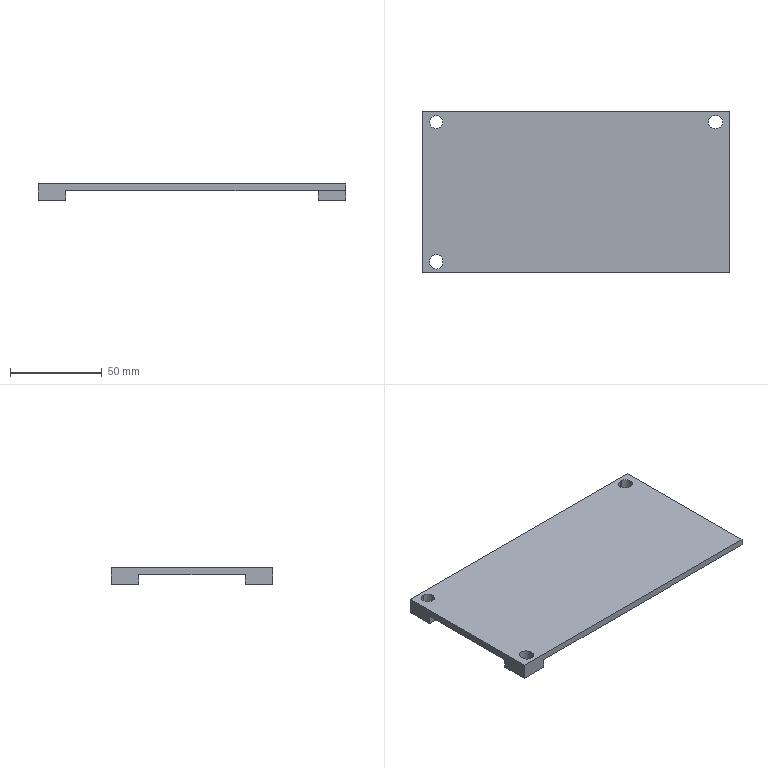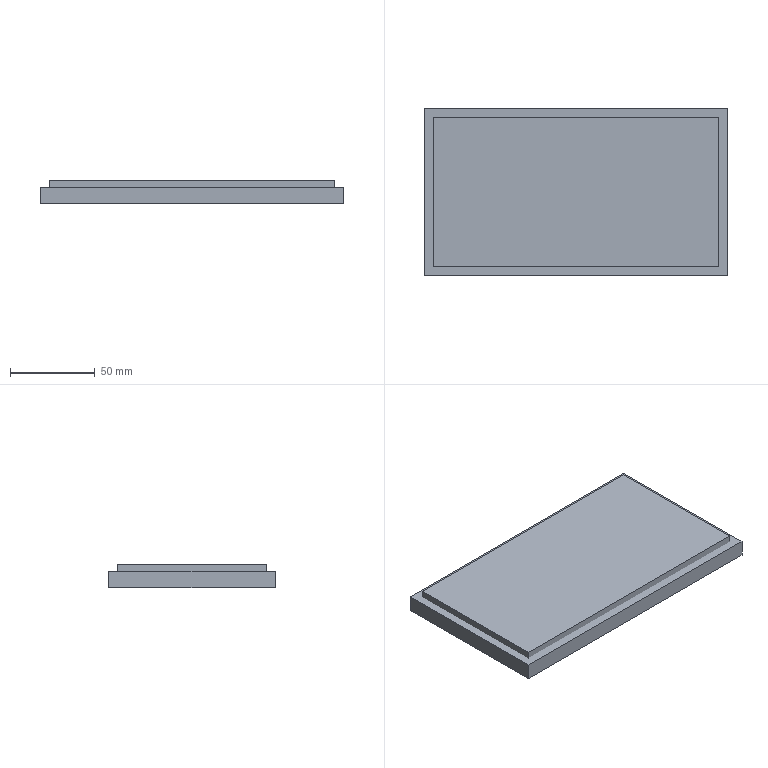CAM job | NX | 3-axis milling | part box 168 x 88.2 x 8.8 mm | stock box 178 x 98.2 x 13.8 mm
Tools:
number,name,description,diameter,corner_radius,flute_length,length,flutes
19,D80,Milling Tool-5 Parameters,80.0,0.0,50.0,75.0,2
14,D10JING,Milling Tool-5 Parameters,10.0,0.0,50.0,75.0,2
15,D10,Milling Tool-5 Parameters,10.0,0.0,50.0,75.0,2
11,D4,Milling Tool-5 Parameters,4.0,0.0,50.0,75.0,2
1,D6A45,Milling Tool-5 Parameters,6.0,0.0,50.0,75.0,2
Operations:
program,operation,operation_type,tool,method,geometry_group,spindle_rpm,surface_speed,feed_per_tooth,feed_cut,feed_plunge,cut_length_mm,path_length_mm,cut_time_min,machine_time_min
1,FLOOR_WALL,VolumeBased25DMillingOperation,D80,METHOD,A,5000.0,1256.0,0.12,1200.0,100.0,852.197,906.197,0.7102,0.7156
1,ADAPTIVE_MILLING,CavityMilling,D10,METHOD,A,9500.0,298.0,0.1579,3000.0,1000.0,3275.989,3347.589,1.094,1.101
1,ZLEVEL_PROFILE_COPY,ZLevelMilling,D10JING,METHOD,A,9500.0,298.0,0.0789,1500.0,1000.0,573.977,648.577,0.3922,0.3997
1,ZLEVEL_PROFILE,ZLevelMilling,D4,METHOD,A,9500.0,119.0,0.1053,2000.0,1000.0,877.237,1307.975,0.4931,0.5361
1,PLANAR_PROFILE,PlanarMilling,D6A45,METHOD,A,9500.0,179.0,0.0789,1500.0,100.0,597.595,1174.58,0.3984,0.4561
2,FLOOR_WALL_COPY,VolumeBased25DMillingOperation,D80,METHOD,B,5000.0,1256.0,0.12,1200.0,100.0,4060.985,5351.556,3.384,3.513
2,FLOOR_WALL_1,VolumeBased25DMillingOperation,D10,METHOD,B,9500.0,0.0,0.0,3000.0,1000.0,14830.073,15089.21,4.956,4.982
2,FLOOR_WALL_1_COPY,VolumeBased25DMillingOperation,D10JING,METHOD,B,9500.0,0.0,0.0737,1400.0,1000.0,3233.981,3677.038,2.317,2.361
2,ZLEVEL_PROFILE_COPY_1,ZLevelMilling,D4,METHOD,B,9500.0,119.0,0.0789,1500.0,1000.0,17.301,81.701,0.0134,0.0198
2,PLANAR_PROFILE_COPY,PlanarMilling,D6A45,METHOD,B,9500.0,179.0,0.0789,1500.0,100.0,288.118,891.476,0.1921,0.2524
2,PLANAR_PROFILE_COPY_COPY,PlanarMilling,D6A45,METHOD,B,9500.0,179.0,0.0789,1500.0,100.0,315.972,681.156,0.2106,0.2472
2,PLANAR_PROFILE_COPY_COPY_COPY,PlanarMilling,D6A45,METHOD,B,9500.0,179.0,0.0789,1500.0,100.0,116.277,185.677,0.0775,0.0845